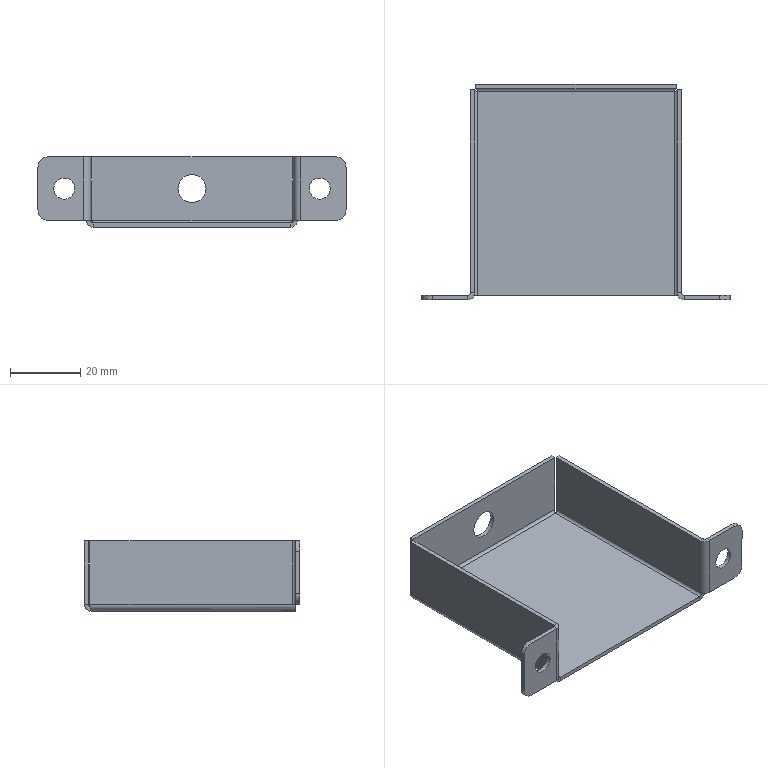Part | SolidWorks | features EdgeFlange 2, Fillet 1, FlatPattern 1, ICE 1, SMBaseFlange 1, SheetMetal 1 | 1 solid | 58 faces | box 87.6 x 61.2 x 20 mm | volume 8600 mm3 | plane 34 | cylinder 20 | spline 4 | commonest cylinder face diameters 6 x8 1.5 x5 3.9 x5 8 x2